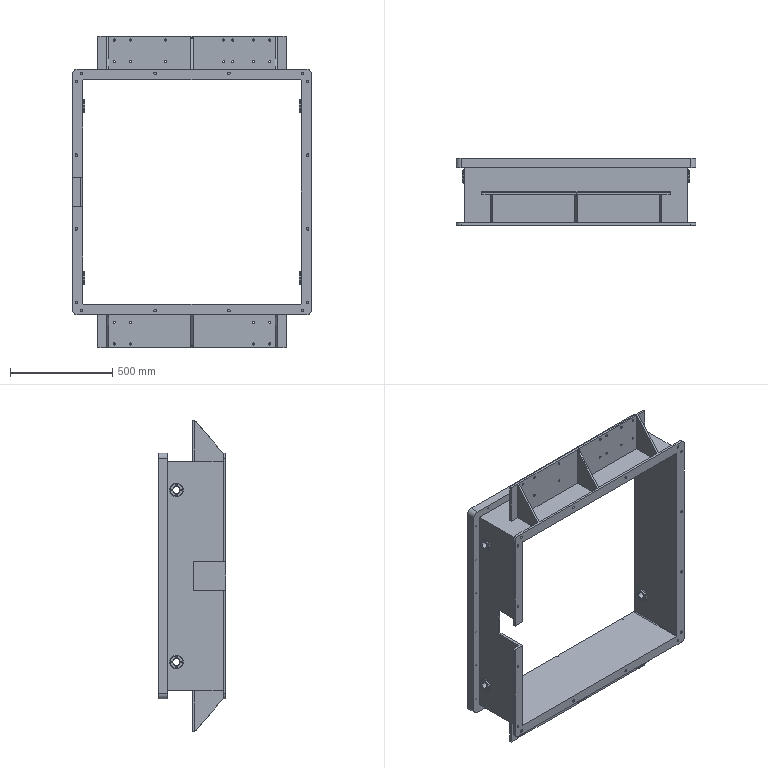Part | NX | features BREP 1 | 1 solid | 477 faces | box 1170 x 328 x 1520 mm | volume 26616083 mm3 | cylinder 252 | cone 128 | plane 81 | torus 16 | commonest cylinder face diameters 5 x64 6.8 x64 10 x44 12 x32 60 x16 8 x10